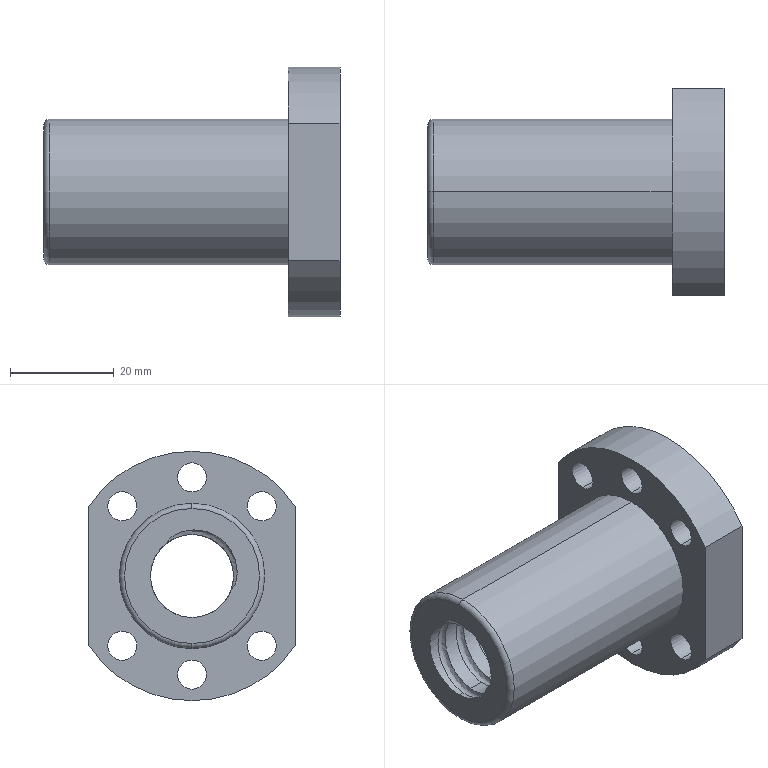Part | STEP file | SHF1605 nut | 1 solid | 50 faces | box 57 x 40 x 48 mm | volume 31691 mm3 | cylinder 42 | plane 5 | torus 2 | spline 1 | commonest cylinder face diameters 16 x25 5.6 x12 48 x3 28 x2